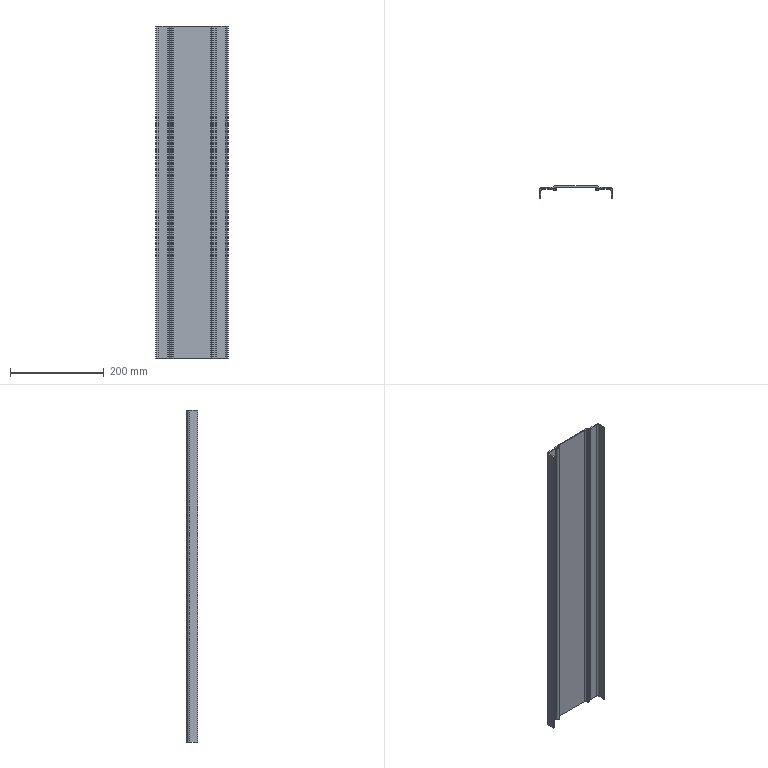Part | STEP file | 1 solid | 52 faces | box 155 x 25 x 709.4 mm | volume 387813 mm3 | cylinder 32 | plane 20 | commonest cylinder face diameters 8 x14 1 x12 3 x4 4.2 x2